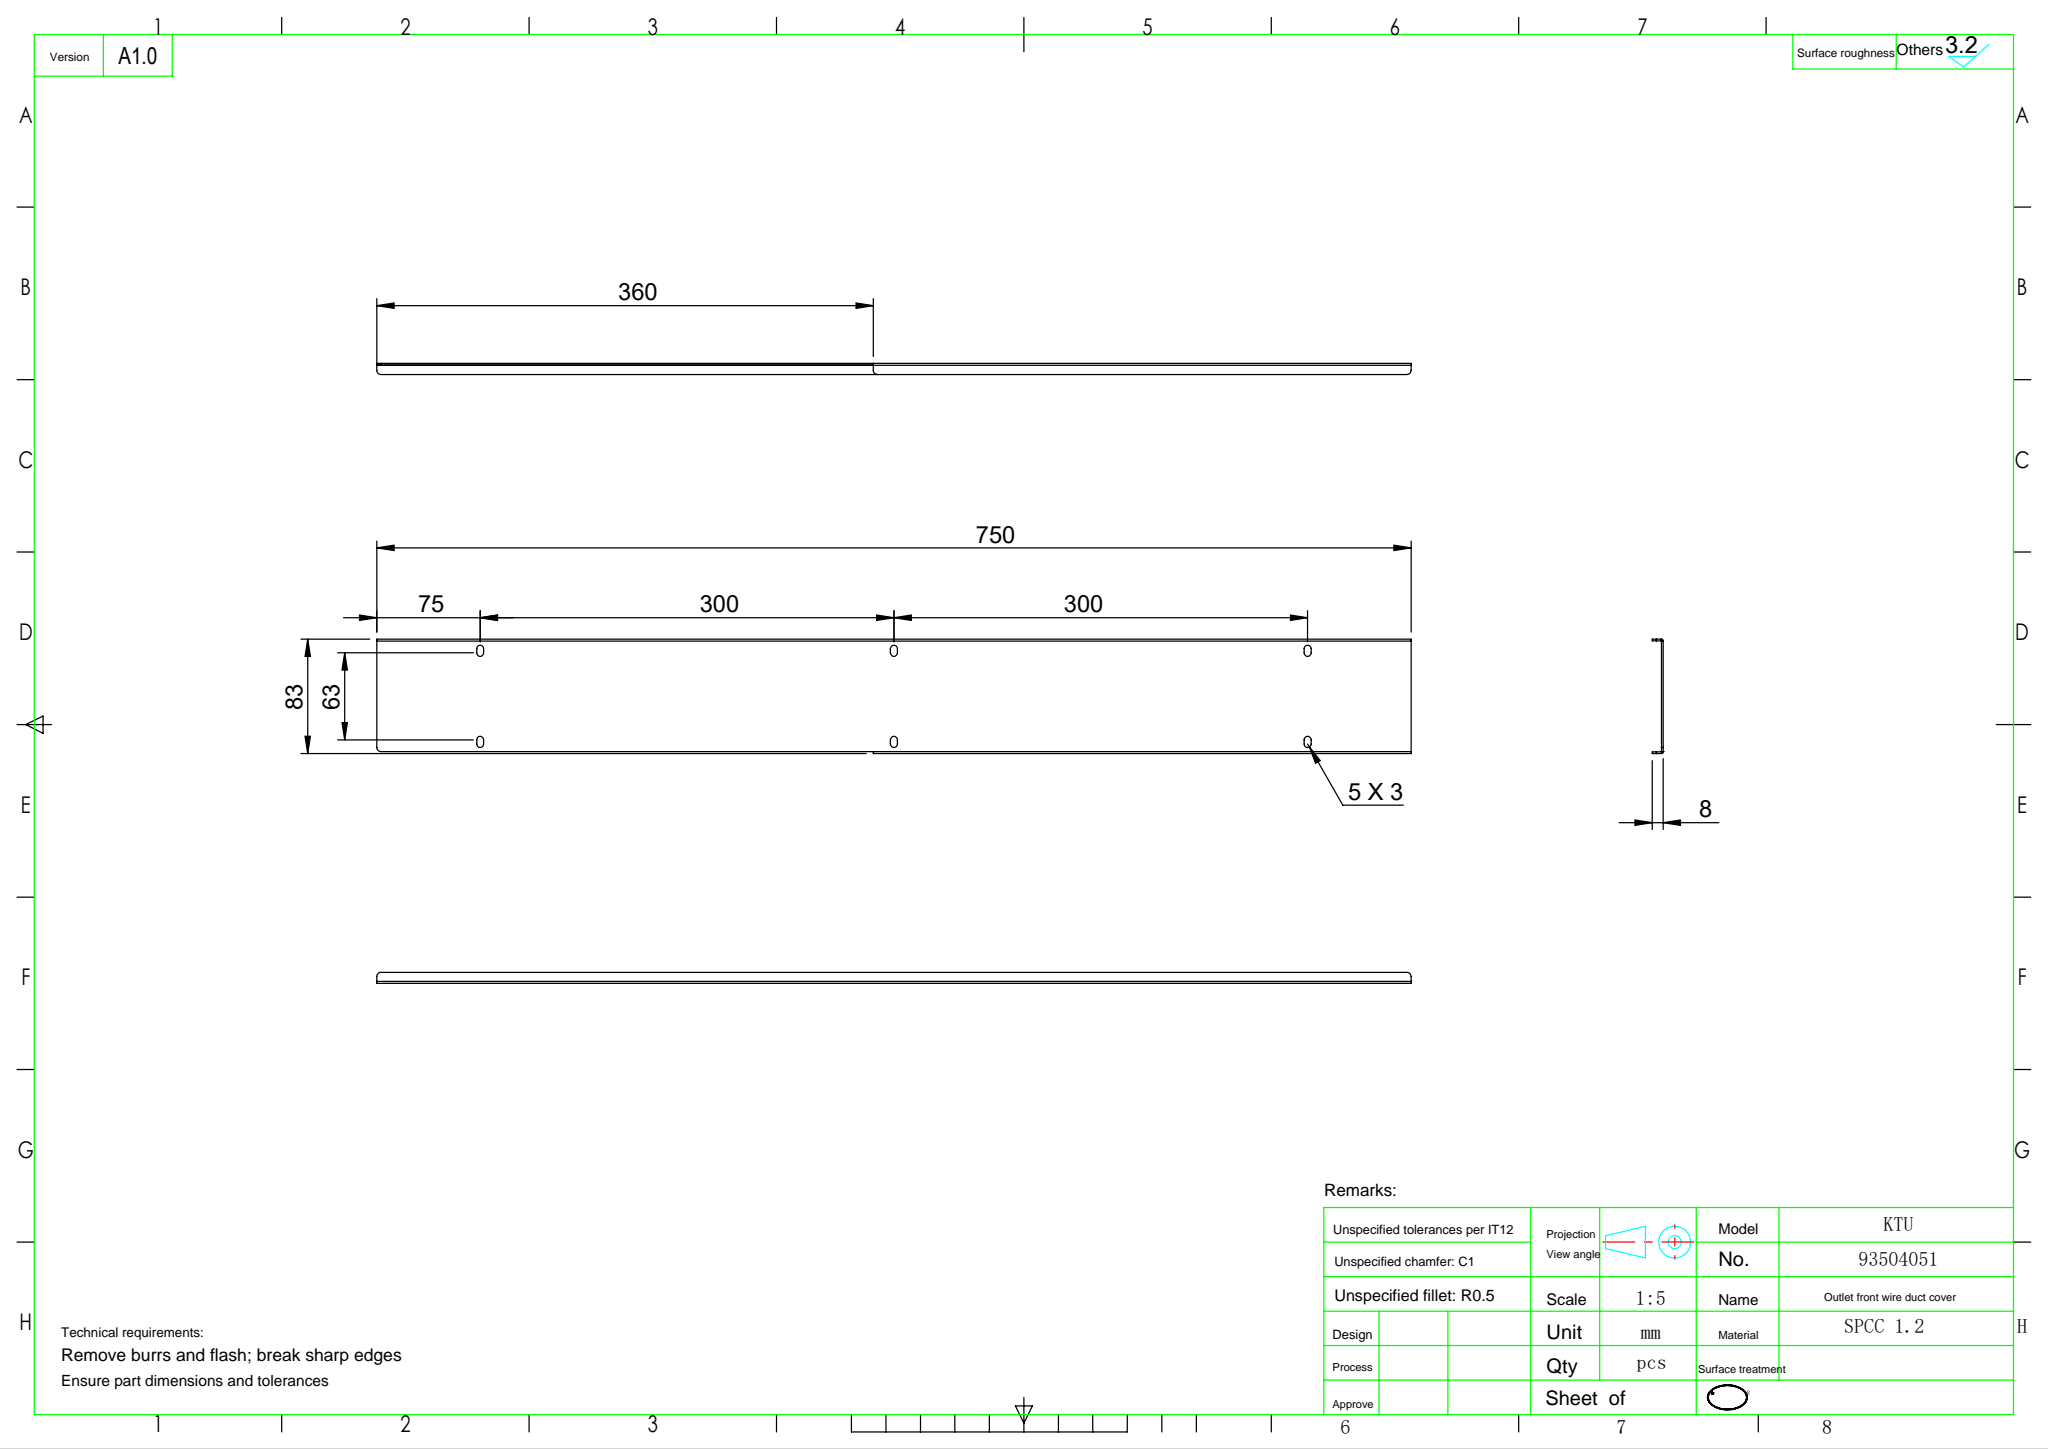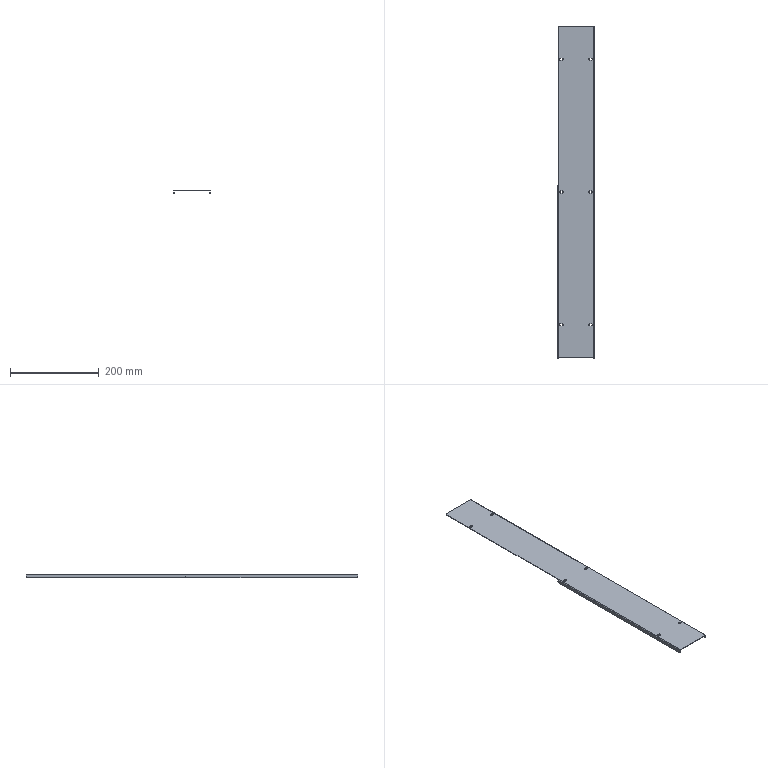Part | SolidWorks | features ICE 2, EdgeFlange 1, Fillet 1, FlatPattern 1, LPattern 1, SMBaseFlange 1, SheetMetal 1 | 1 solid | 57 faces | box 83 x 750 x 8 mm | volume 82624 mm3 | plane 30 | cylinder 27 | commonest cylinder face diameters 5 x18 6 x5 0.4 x2 2.8 x2